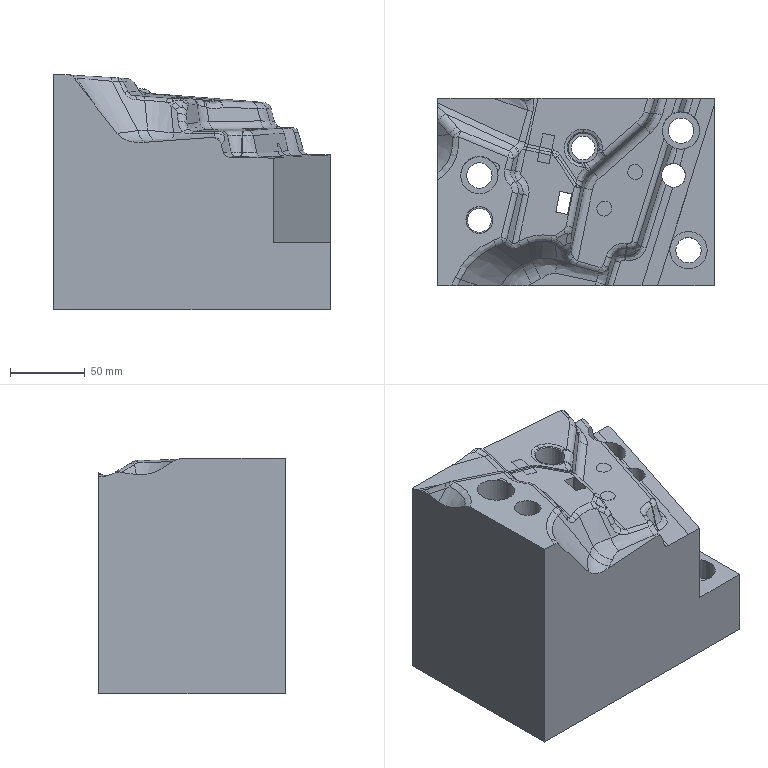Part | NX | features solid 2 | 1 solid | 180 faces | box 185.002 x 125.402 x 157.978 mm | volume 2584355 mm3 | spline 144 | plane 18 | cylinder 18 | commonest cylinder face diameters 1.1 x4 16 x3 17 x3 25 x3 20 x2 18 x1